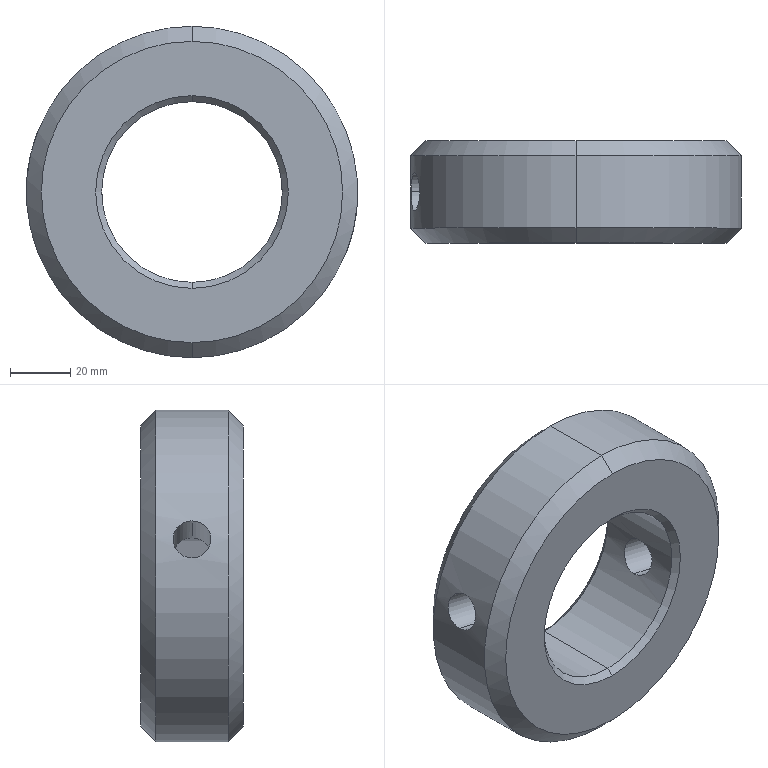Part | SolidWorks | features Chamfer 2, 3DProfileFeature 1, Extrusion 1, HoleWzd 1 | 1 solid | 18 faces | box 110 x 34 x 110 mm | volume 211578 mm3 | cone 8 | cylinder 8 | plane 2 | commonest cylinder face diameters 12.6 x4 60 x2 110 x2
STEP:
#1=CARTESIAN_POINT('',(0.,32.,-30.));
#2=VERTEX_POINT('',#1);
#3=CARTESIAN_POINT('',(0.,32.,30.));
#4=VERTEX_POINT('',#3);
#5=CARTESIAN_POINT('',(0.,32.,0.));
#6=DIRECTION('',(0.,1.,0.));
#7=DIRECTION('',(0.,0.,1.));
#8=AXIS2_PLACEMENT_3D('',#5,#6,#7);
#9=CIRCLE('',#8,30.);
#10=EDGE_CURVE('',#2,#4,#9,.T.);
#11=ORIENTED_EDGE('',*,*,#10,.F.);
#12=CARTESIAN_POINT('',(0.,34.,-32.));
#13=VERTEX_POINT('',#12);
#14=CARTESIAN_POINT('',(0.,32.,-30.));
#15=DIRECTION('',(0.,0.7071,-0.7071));
#16=VECTOR('',#15,1000.);
#17=LINE('',#14,#16);
#18=EDGE_CURVE('',#2,#13,#17,.T.);
#19=ORIENTED_EDGE('',*,*,#18,.T.);
#20=CARTESIAN_POINT('',(0.,34.,32.));
#21=VERTEX_POINT('',#20);
#22=CARTESIAN_POINT('',(0.,34.,0.));
#23=DIRECTION('',(0.,-1.,0.));
#24=DIRECTION('',(0.,0.,1.));
#25=AXIS2_PLACEMENT_3D('',#22,#23,#24);
#26=CIRCLE('',#25,32.);
#27=EDGE_CURVE('',#21,#13,#26,.T.);
#28=ORIENTED_EDGE('',*,*,#27,.F.);
#29=CARTESIAN_POINT('',(0.,32.,30.));
#30=DIRECTION('',(0.,0.7071,0.7071));
#31=VECTOR('',#30,1000.);
#32=LINE('',#29,#31);
#33=EDGE_CURVE('',#4,#21,#32,.T.);
#34=ORIENTED_EDGE('',*,*,#33,.F.);
#35=EDGE_LOOP('',(#11,#19,#28,#34));
#36=FACE_OUTER_BOUND('',#35,.T.);
#37=CARTESIAN_POINT('',(0.,32.,0.));
#38=DIRECTION('',(0.,1.,0.));
#39=DIRECTION('',(0.,0.,1.));
#40=AXIS2_PLACEMENT_3D('',#37,#38,#39);
#41=CONICAL_SURFACE('',#40,30.,0.7854);
#42=ADVANCED_FACE('',(#36),#41,.F.);
#43=CARTESIAN_POINT('',(0.,2.,30.));
#44=VERTEX_POINT('',#43);
#45=CARTESIAN_POINT('',(0.,2.,-30.));
#46=VERTEX_POINT('',#45);
#47=CARTESIAN_POINT('',(0.,2.,0.));
#48=DIRECTION('',(0.,-1.,0.));
#49=DIRECTION('',(0.,0.,1.));
#50=AXIS2_PLACEMENT_3D('',#47,#48,#49);
#51=CIRCLE('',#50,30.);
#52=EDGE_CURVE('',#44,#46,#51,.T.);
#53=ORIENTED_EDGE('',*,*,#52,.F.);
#54=CARTESIAN_POINT('',(0.,0.,32.));
#55=VERTEX_POINT('',#54);
#56=CARTESIAN_POINT('',(0.,0.,32.));
#57=DIRECTION('',(0.,-0.7071,0.7071));
#58=VECTOR('',#57,1000.);
#59=LINE('',#56,#58);
#60=EDGE_CURVE('',#44,#55,#59,.T.);
#61=ORIENTED_EDGE('',*,*,#60,.T.);
#62=CARTESIAN_POINT('',(0.,0.,-32.));
#63=VERTEX_POINT('',#62);
#64=CARTESIAN_POINT('',(0.,0.,0.));
#65=DIRECTION('',(0.,1.,0.));
#66=DIRECTION('',(0.,0.,1.));
#67=AXIS2_PLACEMENT_3D('',#64,#65,#66);
#68=CIRCLE('',#67,32.);
#69=EDGE_CURVE('',#63,#55,#68,.T.);
#70=ORIENTED_EDGE('',*,*,#69,.F.);
#71=CARTESIAN_POINT('',(0.,0.,-32.));
#72=DIRECTION('',(0.,-0.7071,-0.7071));
#73=VECTOR('',#72,1000.);
#74=LINE('',#71,#73);
#75=EDGE_CURVE('',#46,#63,#74,.T.);
#76=ORIENTED_EDGE('',*,*,#75,.F.);
#77=EDGE_LOOP('',(#53,#61,#70,#76));
#78=FACE_OUTER_BOUND('',#77,.T.);
#79=CARTESIAN_POINT('',(0.,0.,0.));
#80=DIRECTION('',(0.,-1.,0.));
#81=DIRECTION('',(0.,0.,-1.));
#82=AXIS2_PLACEMENT_3D('',#79,#80,#81);
#83=CONICAL_SURFACE('',#82,32.,0.7854);
#84=ADVANCED_FACE('',(#78),#83,.F.);
#85=CARTESIAN_POINT('',(0.,34.,50.));
#86=VERTEX_POINT('',#85);
#87=CARTESIAN_POINT('',(0.,34.,-50.));
#88=VERTEX_POINT('',#87);
#89=CARTESIAN_POINT('',(0.,34.,0.));
#90=DIRECTION('',(0.,1.,0.));
#91=DIRECTION('',(0.,0.,1.));
#92=AXIS2_PLACEMENT_3D('',#89,#90,#91);
#93=CIRCLE('',#92,50.);
#94=EDGE_CURVE('',#86,#88,#93,.T.);
#95=ORIENTED_EDGE('',*,*,#94,.F.);
#96=CARTESIAN_POINT('',(0.,29.,55.));
#97=VERTEX_POINT('',#96);
#98=CARTESIAN_POINT('',(0.,34.,50.));
#99=DIRECTION('',(0.,-0.7071,0.7071));
#100=VECTOR('',#99,1000.);
#101=LINE('',#98,#100);
#102=EDGE_CURVE('',#86,#97,#101,.T.);
#103=ORIENTED_EDGE('',*,*,#102,.T.);
#104=CARTESIAN_POINT('',(0.,29.,-55.));
#105=VERTEX_POINT('',#104);
#106=CARTESIAN_POINT('',(0.,29.,0.));
#107=DIRECTION('',(0.,-1.,0.));
#108=DIRECTION('',(0.,0.,1.));
#109=AXIS2_PLACEMENT_3D('',#106,#107,#108);
#110=CIRCLE('',#109,55.);
#111=EDGE_CURVE('',#105,#97,#110,.T.);
#112=ORIENTED_EDGE('',*,*,#111,.F.);
#113=CARTESIAN_POINT('',(0.,34.,-50.));
#114=DIRECTION('',(0.,-0.7071,-0.7071));
#115=VECTOR('',#114,1000.);
#116=LINE('',#113,#115);
#117=EDGE_CURVE('',#88,#105,#116,.T.);
#118=ORIENTED_EDGE('',*,*,#117,.F.);
#119=EDGE_LOOP('',(#95,#103,#112,#118));
#120=FACE_OUTER_BOUND('',#119,.T.);
#121=CARTESIAN_POINT('',(0.,34.,0.));
#122=DIRECTION('',(0.,-1.,0.));
#123=DIRECTION('',(0.,0.,-1.));
#124=AXIS2_PLACEMENT_3D('',#121,#122,#123);
#125=CONICAL_SURFACE('',#124,50.,0.7854);
#126=ADVANCED_FACE('',(#120),#125,.T.);
#127=CARTESIAN_POINT('',(0.,0.,-50.));
#128=VERTEX_POINT('',#127);
#129=CARTESIAN_POINT('',(0.,0.,50.));
#130=VERTEX_POINT('',#129);
#131=CARTESIAN_POINT('',(0.,0.,0.));
#132=DIRECTION('',(0.,-1.,0.));
#133=DIRECTION('',(0.,0.,1.));
#134=AXIS2_PLACEMENT_3D('',#131,#132,#133);
#135=CIRCLE('',#134,50.);
#136=EDGE_CURVE('',#128,#130,#135,.T.);
#137=ORIENTED_EDGE('',*,*,#136,.F.);
#138=CARTESIAN_POINT('',(0.,5.,-55.));
#139=VERTEX_POINT('',#138);
#140=CARTESIAN_POINT('',(0.,5.,-55.));
#141=DIRECTION('',(0.,0.7071,-0.7071));
#142=VECTOR('',#141,1000.);
#143=LINE('',#140,#142);
#144=EDGE_CURVE('',#128,#139,#143,.T.);
#145=ORIENTED_EDGE('',*,*,#144,.T.);
#146=CARTESIAN_POINT('',(0.,5.,55.));
#147=VERTEX_POINT('',#146);
#148=CARTESIAN_POINT('',(0.,5.,0.));
#149=DIRECTION('',(0.,1.,0.));
#150=DIRECTION('',(0.,0.,1.));
#151=AXIS2_PLACEMENT_3D('',#148,#149,#150);
#152=CIRCLE('',#151,55.);
#153=EDGE_CURVE('',#147,#139,#152,.T.);
#154=ORIENTED_EDGE('',*,*,#153,.F.);
#155=CARTESIAN_POINT('',(0.,5.,55.));
#156=DIRECTION('',(0.,0.7071,0.7071));
#157=VECTOR('',#156,1000.);
#158=LINE('',#155,#157);
#159=EDGE_CURVE('',#130,#147,#158,.T.);
#160=ORIENTED_EDGE('',*,*,#159,.F.);
#161=EDGE_LOOP('',(#137,#145,#154,#160));
#162=FACE_OUTER_BOUND('',#161,.T.);
#163=CARTESIAN_POINT('',(0.,5.,0.));
#164=DIRECTION('',(0.,1.,0.));
#165=DIRECTION('',(0.,0.,1.));
#166=AXIS2_PLACEMENT_3D('',#163,#164,#165);
#167=CONICAL_SURFACE('',#166,55.,0.7854);
#168=ADVANCED_FACE('',(#162),#167,.T.);
#169=CARTESIAN_POINT('',(-51.87,17.,18.289));
#170=VERTEX_POINT('',#169);
#171=CARTESIAN_POINT('',(-54.671,17.,6.005));
#172=VERTEX_POINT('',#171);
#173=CARTESIAN_POINT('',(-51.87,17.,18.289));
#174=CARTESIAN_POINT('',(-51.87,16.589,18.289));
#175=CARTESIAN_POINT('',(-51.883,16.18,18.252));
#176=CARTESIAN_POINT('',(-51.924,15.57,18.137));
#177=CARTESIAN_POINT('',(-51.94,15.368,18.088));
#178=CARTESIAN_POINT('',(-51.98,14.973,17.975));
#179=CARTESIAN_POINT('',(-52.025,14.586,17.843));
#180=CARTESIAN_POINT('',(-52.082,14.215,17.676));
#181=CARTESIAN_POINT('',(-52.145,13.851,17.491));
#182=CARTESIAN_POINT('',(-52.179,13.672,17.389));
#183=CARTESIAN_POINT('',(-52.288,13.156,17.06));
#184=CARTESIAN_POINT('',(-52.369,12.839,16.811));
#185=CARTESIAN_POINT('',(-52.544,12.258,16.256));
#186=CARTESIAN_POINT('',(-52.639,11.992,15.946));
#187=CARTESIAN_POINT('',(-52.834,11.534,15.288));
#188=CARTESIAN_POINT('',(-52.933,11.341,14.94));
#189=CARTESIAN_POINT('',(-53.085,11.103,14.388));
#190=CARTESIAN_POINT('',(-53.136,11.032,14.198));
#191=CARTESIAN_POINT('',(-53.237,10.912,13.815));
#192=CARTESIAN_POINT('',(-53.287,10.862,13.622));
#193=CARTESIAN_POINT('',(-53.434,10.741,13.036));
#194=CARTESIAN_POINT('',(-53.53,10.7,12.638));
#195=CARTESIAN_POINT('',(-53.715,10.7,11.826));
#196=CARTESIAN_POINT('',(-53.802,10.74,11.426));
#197=CARTESIAN_POINT('',(-53.923,10.86,10.833));
#198=CARTESIAN_POINT('',(-53.962,10.91,10.637));
#199=CARTESIAN_POINT('',(-54.037,11.03,10.249));
#200=CARTESIAN_POINT('',(-54.073,11.1,10.055));
#201=CARTESIAN_POINT('',(-54.176,11.337,9.491));
#202=CARTESIAN_POINT('',(-54.237,11.53,9.134));
#203=CARTESIAN_POINT('',(-54.347,11.986,8.457));
#204=CARTESIAN_POINT('',(-54.396,12.252,8.136));
#205=CARTESIAN_POINT('',(-54.479,12.832,7.559));
#206=CARTESIAN_POINT('',(-54.514,13.149,7.299));
#207=CARTESIAN_POINT('',(-54.559,13.665,6.955));
#208=CARTESIAN_POINT('',(-54.572,13.844,6.848));
#209=CARTESIAN_POINT('',(-54.596,14.207,6.654));
#210=CARTESIAN_POINT('',(-54.607,14.392,6.566));
#211=CARTESIAN_POINT('',(-54.635,14.961,6.33));
#212=CARTESIAN_POINT('',(-54.649,15.357,6.209));
#213=CARTESIAN_POINT('',(-54.667,16.172,6.046));
#214=CARTESIAN_POINT('',(-54.671,16.583,6.005));
#215=CARTESIAN_POINT('',(-54.671,17.,6.005));
#216=B_SPLINE_CURVE_WITH_KNOTS('',3,(#173,#174,#175,#176,#177,#178,#179,#180,#181,#182,#183,#184,#185,#186,#187,#188,#189,#190,#191,#192,#193,#194,#195,#196,#197,#198,#199,#200,#201,#202,#203,#204,#205,#206,#207,#208,#209,#210,#211,#212,#213,#214,#215),.UNSPECIFIED.,.F.,.F.,(4,2,2,1,2,2,2,2,2,2,2,2,2,2,2,2,2,2,2,2,2,4),(0.01971,0.02094,0.02156,0.02218,0.02279,0.02341,0.02464,0.02587,0.0271,0.02772,0.02834,0.02957,0.0308,0.03141,0.03203,0.03326,0.03449,0.03573,0.03634,0.03696,0.03819,0.03942),.UNSPECIFIED.);
#217=EDGE_CURVE('',#170,#172,#216,.T.);
#218=ORIENTED_EDGE('',*,*,#217,.F.);
#219=CARTESIAN_POINT('',(-27.196,17.,12.663));
#220=VERTEX_POINT('',#219);
#221=CARTESIAN_POINT('',(55.024,17.,-6.085));
#222=DIRECTION('',(0.975,0.,-0.2223));
#223=VECTOR('',#222,1000.);
#224=LINE('',#221,#223);
#225=EDGE_CURVE('',#170,#220,#224,.T.);
#226=ORIENTED_EDGE('',*,*,#225,.T.);
#227=CARTESIAN_POINT('',(-29.998,17.,0.3785));
#228=VERTEX_POINT('',#227);
#229=CARTESIAN_POINT('',(-27.196,17.,12.663));
#230=CARTESIAN_POINT('',(-27.196,16.588,12.663));
#231=CARTESIAN_POINT('',(-27.214,16.178,12.626));
#232=CARTESIAN_POINT('',(-27.283,15.362,12.475));
#233=CARTESIAN_POINT('',(-27.335,14.966,12.363));
#234=CARTESIAN_POINT('',(-27.432,14.397,12.144));
#235=CARTESIAN_POINT('',(-27.469,14.212,12.062));
#236=CARTESIAN_POINT('',(-27.548,13.847,11.88));
#237=CARTESIAN_POINT('',(-27.591,13.669,11.78));
#238=CARTESIAN_POINT('',(-27.727,13.155,11.458));
#239=CARTESIAN_POINT('',(-27.827,12.838,11.215));
#240=CARTESIAN_POINT('',(-28.041,12.257,10.668));
#241=CARTESIAN_POINT('',(-28.155,11.992,10.363));
#242=CARTESIAN_POINT('',(-28.385,11.536,9.716));
#243=CARTESIAN_POINT('',(-28.501,11.342,9.372));
#244=CARTESIAN_POINT('',(-28.674,11.103,8.823));
#245=CARTESIAN_POINT('',(-28.731,11.033,8.635));
#246=CARTESIAN_POINT('',(-28.843,10.913,8.255));
#247=CARTESIAN_POINT('',(-28.951,10.812,7.871));
#248=CARTESIAN_POINT('',(-29.054,10.752,7.477));
#249=CARTESIAN_POINT('',(-29.154,10.711,7.078));
#250=CARTESIAN_POINT('',(-29.202,10.7,6.875));
#251=CARTESIAN_POINT('',(-29.341,10.7,6.267));
#252=CARTESIAN_POINT('',(-29.424,10.74,5.866));
#253=CARTESIAN_POINT('',(-29.571,10.901,5.071));
#254=CARTESIAN_POINT('',(-29.636,11.023,4.673));
#255=CARTESIAN_POINT('',(-29.746,11.338,3.918));
#256=CARTESIAN_POINT('',(-29.79,11.531,3.557));
#257=CARTESIAN_POINT('',(-29.846,11.875,3.042));
#258=CARTESIAN_POINT('',(-29.862,11.999,2.874));
#259=CARTESIAN_POINT('',(-29.892,12.26,2.554));
#260=CARTESIAN_POINT('',(-29.904,12.398,2.401));
#261=CARTESIAN_POINT('',(-29.937,12.832,1.963));
#262=CARTESIAN_POINT('',(-29.953,13.149,1.698));
#263=CARTESIAN_POINT('',(-29.976,13.838,1.23));
#264=CARTESIAN_POINT('',(-29.983,14.2,1.033));
#265=CARTESIAN_POINT('',(-29.99,14.769,0.792));
#266=CARTESIAN_POINT('',(-29.991,14.962,0.7208));
#267=CARTESIAN_POINT('',(-29.994,15.358,0.5974));
#268=CARTESIAN_POINT('',(-29.995,15.561,0.5451));
#269=CARTESIAN_POINT('',(-29.997,16.171,0.4206));
#270=CARTESIAN_POINT('',(-29.998,16.583,0.3785));
#271=CARTESIAN_POINT('',(-29.998,17.,0.3785));
#272=B_SPLINE_CURVE_WITH_KNOTS('',3,(#229,#230,#231,#232,#233,#234,#235,#236,#237,#238,#239,#240,#241,#242,#243,#244,#245,#246,#247,#248,#249,#250,#251,#252,#253,#254,#255,#256,#257,#258,#259,#260,#261,#262,#263,#264,#265,#266,#267,#268,#269,#270,#271),.UNSPECIFIED.,.F.,.F.,(4,2,2,2,2,2,2,2,2,1,2,2,2,2,2,2,2,2,2,2,2,4),(0.01975,0.02099,0.02222,0.02284,0.02345,0.02469,0.02592,0.02716,0.02777,0.02839,0.02901,0.02962,0.03086,0.03209,0.03333,0.03394,0.03456,0.0358,0.03703,0.03765,0.03826,0.0395),.UNSPECIFIED.);
#273=EDGE_CURVE('',#220,#228,#272,.T.);
#274=ORIENTED_EDGE('',*,*,#273,.T.);
#275=CARTESIAN_POINT('',(52.223,17.,-18.37));
#276=DIRECTION('',(0.975,0.,-0.2223));
#277=VECTOR('',#276,1000.);
#278=LINE('',#275,#277);
#279=EDGE_CURVE('',#172,#228,#278,.T.);
#280=ORIENTED_EDGE('',*,*,#279,.F.);
#281=EDGE_LOOP('',(#218,#226,#274,#280));
#282=FACE_OUTER_BOUND('',#281,.T.);
#283=CARTESIAN_POINT('',(53.624,17.,-12.228));
#284=DIRECTION('',(0.975,0.,-0.2223));
#285=DIRECTION('',(-0.2223,0.,-0.975));
#286=AXIS2_PLACEMENT_3D('',#283,#284,#285);
#287=CYLINDRICAL_SURFACE('',#286,6.3);
#288=ADVANCED_FACE('',(#282),#287,.F.);
#289=CARTESIAN_POINT('',(27.196,17.,-12.663));
#290=VERTEX_POINT('',#289);
#291=CARTESIAN_POINT('',(29.998,17.,-0.3785));
#292=VERTEX_POINT('',#291);
#293=CARTESIAN_POINT('',(27.196,17.,-12.663));
#294=CARTESIAN_POINT('',(27.196,16.582,-12.663));
#295=CARTESIAN_POINT('',(27.214,16.172,-12.625));
#296=CARTESIAN_POINT('',(27.266,15.567,-12.513));
#297=CARTESIAN_POINT('',(27.287,15.367,-12.467));
#298=CARTESIAN_POINT('',(27.338,14.971,-12.355));
#299=CARTESIAN_POINT('',(27.368,14.774,-12.289));
#300=CARTESIAN_POINT('',(27.466,14.202,-12.068));
#301=CARTESIAN_POINT('',(27.545,13.841,-11.887));
#302=CARTESIAN_POINT('',(27.726,13.157,-11.46));
#303=CARTESIAN_POINT('',(27.828,12.834,-11.211));
#304=CARTESIAN_POINT('',(28.042,12.255,-10.665));
#305=CARTESIAN_POINT('',(28.154,11.994,-10.366));
#306=CARTESIAN_POINT('',(28.386,11.534,-9.713));
#307=CARTESIAN_POINT('',(28.503,11.339,-9.365));
#308=CARTESIAN_POINT('',(28.674,11.103,-8.822));
#309=CARTESIAN_POINT('',(28.731,11.033,-8.636));
#310=CARTESIAN_POINT('',(28.842,10.913,-8.256));
#311=CARTESIAN_POINT('',(28.897,10.862,-8.061));
#312=CARTESIAN_POINT('',(29.058,10.74,-7.471));
#313=CARTESIAN_POINT('',(29.157,10.7,-7.074));
#314=CARTESIAN_POINT('',(29.34,10.7,-6.27));
#315=CARTESIAN_POINT('',(29.425,10.741,-5.86));
#316=CARTESIAN_POINT('',(29.572,10.903,-5.064));
#317=CARTESIAN_POINT('',(29.636,11.022,-4.675));
#318=CARTESIAN_POINT('',(29.718,11.26,-4.106));
#319=CARTESIAN_POINT('',(29.744,11.349,-3.918));
#320=CARTESIAN_POINT('',(29.789,11.544,-3.555));
#321=CARTESIAN_POINT('',(29.81,11.65,-3.379));
#322=CARTESIAN_POINT('',(29.865,11.991,-2.868));
#323=CARTESIAN_POINT('',(29.893,12.253,-2.547));
#324=CARTESIAN_POINT('',(29.938,12.839,-1.957));
#325=CARTESIAN_POINT('',(29.953,13.155,-1.694));
#326=CARTESIAN_POINT('',(29.97,13.666,-1.347));
#327=CARTESIAN_POINT('',(29.975,13.843,-1.239));
#328=CARTESIAN_POINT('',(29.982,14.208,-1.04));
#329=CARTESIAN_POINT('',(29.985,14.396,-0.9496));
#330=CARTESIAN_POINT('',(29.992,14.967,-0.7083));
#331=CARTESIAN_POINT('',(29.994,15.36,-0.5862));
#332=CARTESIAN_POINT('',(29.996,15.967,-0.4621));
#333=CARTESIAN_POINT('',(29.997,16.174,-0.4306));
#334=CARTESIAN_POINT('',(29.997,16.588,-0.3888));
#335=CARTESIAN_POINT('',(29.998,16.794,-0.3785));
#336=CARTESIAN_POINT('',(29.998,17.,-0.3785));
#337=B_SPLINE_CURVE_WITH_KNOTS('',3,(#293,#294,#295,#296,#297,#298,#299,#300,#301,#302,#303,#304,#305,#306,#307,#308,#309,#310,#311,#312,#313,#314,#315,#316,#317,#318,#319,#320,#321,#322,#323,#324,#325,#326,#327,#328,#329,#330,#331,#332,#333,#334,#335,#336),.UNSPECIFIED.,.F.,.F.,(4,2,2,2,2,2,2,2,2,2,2,2,2,2,2,2,2,2,2,2,2,4),(0.,0.001234,0.001852,0.002469,0.003703,0.004938,0.006172,0.007407,0.008024,0.008641,0.009876,0.01111,0.01234,0.01296,0.01358,0.01481,0.01605,0.01667,0.01728,0.01852,0.01913,0.01975),.UNSPECIFIED.);
#338=EDGE_CURVE('',#290,#292,#337,.T.);
#339=ORIENTED_EDGE('',*,*,#338,.T.);
#340=CARTESIAN_POINT('',(54.671,17.,-6.005));
#341=VERTEX_POINT('',#340);
#342=CARTESIAN_POINT('',(55.024,17.,-6.085));
#343=DIRECTION('',(0.975,0.,-0.2223));
#344=VECTOR('',#343,1000.);
#345=LINE('',#342,#344);
#346=EDGE_CURVE('',#292,#341,#345,.T.);
#347=ORIENTED_EDGE('',*,*,#346,.T.);
#348=CARTESIAN_POINT('',(51.87,17.,-18.289));
#349=VERTEX_POINT('',#348);
#350=CARTESIAN_POINT('',(51.87,17.,-18.289));
#351=CARTESIAN_POINT('',(51.87,16.583,-18.289));
#352=CARTESIAN_POINT('',(51.884,16.174,-18.251));
#353=CARTESIAN_POINT('',(51.924,15.569,-18.136));
#354=CARTESIAN_POINT('',(51.94,15.37,-18.089));
#355=CARTESIAN_POINT('',(51.98,14.974,-17.975));
#356=CARTESIAN_POINT('',(52.003,14.777,-17.908));
#357=CARTESIAN_POINT('',(52.08,14.205,-17.682));
#358=CARTESIAN_POINT('',(52.143,13.843,-17.498));
#359=CARTESIAN_POINT('',(52.287,13.159,-17.062));
#360=CARTESIAN_POINT('',(52.37,12.835,-16.808));
#361=CARTESIAN_POINT('',(52.545,12.254,-16.252));
#362=CARTESIAN_POINT('',(52.638,11.993,-15.948));
#363=CARTESIAN_POINT('',(52.785,11.648,-15.452));
#364=CARTESIAN_POINT('',(52.835,11.541,-15.28));
#365=CARTESIAN_POINT('',(52.935,11.347,-14.93));
#366=CARTESIAN_POINT('',(53.036,11.171,-14.572));
#367=CARTESIAN_POINT('',(53.136,11.032,-14.198));
#368=CARTESIAN_POINT('',(53.237,10.912,-13.816));
#369=CARTESIAN_POINT('',(53.287,10.862,-13.62));
#370=CARTESIAN_POINT('',(53.436,10.74,-13.029));
#371=CARTESIAN_POINT('',(53.532,10.7,-12.631));
#372=CARTESIAN_POINT('',(53.715,10.7,-11.829));
#373=CARTESIAN_POINT('',(53.803,10.741,-11.42));
#374=CARTESIAN_POINT('',(53.965,10.902,-10.628));
#375=CARTESIAN_POINT('',(54.039,11.021,-10.242));
#376=CARTESIAN_POINT('',(54.142,11.258,-9.679));
#377=CARTESIAN_POINT('',(54.175,11.347,-9.492));
#378=CARTESIAN_POINT('',(54.237,11.542,-9.133));
#379=CARTESIAN_POINT('',(54.266,11.648,-8.958));
#380=CARTESIAN_POINT('',(54.348,11.99,-8.452));
#381=CARTESIAN_POINT('',(54.396,12.251,-8.137));
#382=CARTESIAN_POINT('',(54.48,12.839,-7.553));
#383=CARTESIAN_POINT('',(54.515,13.157,-7.294));
#384=CARTESIAN_POINT('',(54.559,13.668,-6.953));
#385=CARTESIAN_POINT('',(54.572,13.844,-6.847));
#386=CARTESIAN_POINT('',(54.596,14.209,-6.652));
#387=CARTESIAN_POINT('',(54.607,14.398,-6.563));
#388=CARTESIAN_POINT('',(54.635,14.97,-6.327));
#389=CARTESIAN_POINT('',(54.649,15.363,-6.207));
#390=CARTESIAN_POINT('',(54.667,16.171,-6.046));
#391=CARTESIAN_POINT('',(54.671,16.589,-6.005));
#392=CARTESIAN_POINT('',(54.671,17.,-6.005));
#393=B_SPLINE_CURVE_WITH_KNOTS('',3,(#350,#351,#352,#353,#354,#355,#356,#357,#358,#359,#360,#361,#362,#363,#364,#365,#366,#367,#368,#369,#370,#371,#372,#373,#374,#375,#376,#377,#378,#379,#380,#381,#382,#383,#384,#385,#386,#387,#388,#389,#390,#391,#392),.UNSPECIFIED.,.F.,.F.,(4,2,2,2,2,2,2,2,1,2,2,2,2,2,2,2,2,2,2,2,2,4),(0.,0.001232,0.001848,0.002464,0.003696,0.004928,0.00616,0.006776,0.007392,0.008008,0.008624,0.009856,0.01109,0.01232,0.01294,0.01355,0.01478,0.01602,0.01663,0.01725,0.01848,0.01971),.UNSPECIFIED.);
#394=EDGE_CURVE('',#349,#341,#393,.T.);
#395=ORIENTED_EDGE('',*,*,#394,.F.);
#396=CARTESIAN_POINT('',(52.223,17.,-18.37));
#397=DIRECTION('',(0.975,0.,-0.2223));
#398=VECTOR('',#397,1000.);
#399=LINE('',#396,#398);
#400=EDGE_CURVE('',#290,#349,#399,.T.);
#401=ORIENTED_EDGE('',*,*,#400,.F.);
#402=EDGE_LOOP('',(#339,#347,#395,#401));
#403=FACE_OUTER_BOUND('',#402,.T.);
#404=CARTESIAN_POINT('',(53.624,17.,-12.228));
#405=DIRECTION('',(0.975,0.,-0.2223));
#406=DIRECTION('',(-0.2223,0.,-0.975));
#407=AXIS2_PLACEMENT_3D('',#404,#405,#406);
#408=CYLINDRICAL_SURFACE('',#407,6.3);
#409=ADVANCED_FACE('',(#403),#408,.F.);
#410=CARTESIAN_POINT('',(-29.998,17.,0.3785));
#411=CARTESIAN_POINT('',(-29.998,17.418,0.3785));
#412=CARTESIAN_POINT('',(-29.997,17.828,0.4206));
#413=CARTESIAN_POINT('',(-29.995,18.433,0.5438));
#414=CARTESIAN_POINT('',(-29.994,18.633,0.5949));
#415=CARTESIAN_POINT('',(-29.991,19.029,0.7178));
#416=CARTESIAN_POINT('',(-29.99,19.226,0.7898));
#417=CARTESIAN_POINT('',(-29.983,19.798,1.032));
#418=CARTESIAN_POINT('',(-29.976,20.159,1.229));
#419=CARTESIAN_POINT('',(-29.953,20.843,1.693));
#420=CARTESIAN_POINT('',(-29.937,21.166,1.961));
#421=CARTESIAN_POINT('',(-29.893,21.745,2.546));
#422=CARTESIAN_POINT('',(-29.865,22.006,2.864));
#423=CARTESIAN_POINT('',(-29.791,22.466,3.553));
#424=CARTESIAN_POINT('',(-29.746,22.661,3.917));
#425=CARTESIAN_POINT('',(-29.664,22.897,4.481));
#426=CARTESIAN_POINT('',(-29.635,22.967,4.673));
#427=CARTESIAN_POINT('',(-29.57,23.087,5.063));
#428=CARTESIAN_POINT('',(-29.535,23.138,5.263));
#429=CARTESIAN_POINT('',(-29.424,23.26,5.864));
#430=CARTESIAN_POINT('',(-29.341,23.3,6.265));
#431=CARTESIAN_POINT('',(-29.158,23.3,7.069));
#432=CARTESIAN_POINT('',(-29.057,23.259,7.475));
#433=CARTESIAN_POINT('',(-28.844,23.097,8.257));
#434=CARTESIAN_POINT('',(-28.733,22.978,8.635));
#435=CARTESIAN_POINT('',(-28.56,22.74,9.183));
#436=CARTESIAN_POINT('',(-28.502,22.651,9.364));
#437=CARTESIAN_POINT('',(-28.386,22.456,9.71));
#438=CARTESIAN_POINT('',(-28.328,22.35,9.877));
#439=CARTESIAN_POINT('',(-28.156,22.009,10.362));
#440=CARTESIAN_POINT('',(-28.042,21.747,10.664));
#441=CARTESIAN_POINT('',(-27.826,21.161,11.215));
#442=CARTESIAN_POINT('',(-27.726,20.845,11.459));
#443=CARTESIAN_POINT('',(-27.591,20.334,11.779));
#444=CARTESIAN_POINT('',(-27.549,20.157,11.878));
#445=CARTESIAN_POINT('',(-27.469,19.792,12.06));
#446=CARTESIAN_POINT('',(-27.433,19.604,12.143));
#447=CARTESIAN_POINT('',(-27.334,19.033,12.364));
#448=CARTESIAN_POINT('',(-27.284,18.64,12.475));
#449=CARTESIAN_POINT('',(-27.232,18.033,12.587));
#450=CARTESIAN_POINT('',(-27.218,17.826,12.616));
#451=CARTESIAN_POINT('',(-27.201,17.412,12.654));
#452=CARTESIAN_POINT('',(-27.196,17.206,12.663));
#453=CARTESIAN_POINT('',(-27.196,17.,12.663));
#454=B_SPLINE_CURVE_WITH_KNOTS('',3,(#410,#411,#412,#413,#414,#415,#416,#417,#418,#419,#420,#421,#422,#423,#424,#425,#426,#427,#428,#429,#430,#431,#432,#433,#434,#435,#436,#437,#438,#439,#440,#441,#442,#443,#444,#445,#446,#447,#448,#449,#450,#451,#452,#453),.UNSPECIFIED.,.F.,.F.,(4,2,2,2,2,2,2,2,2,2,2,2,2,2,2,2,2,2,2,2,2,4),(0.,0.001234,0.001852,0.002469,0.003703,0.004938,0.006172,0.007407,0.008024,0.008641,0.009876,0.01111,0.01234,0.01296,0.01358,0.01481,0.01605,0.01667,0.01728,0.01852,0.01913,0.01975),.UNSPECIFIED.);
#455=EDGE_CURVE('',#228,#220,#454,.T.);
#456=ORIENTED_EDGE('',*,*,#455,.F.);
#457=ORIENTED_EDGE('',*,*,#273,.F.);
#458=EDGE_LOOP('',(#456,#457));
#459=FACE_BOUND('',#458,.T.);
#460=ORIENTED_EDGE('',*,*,#10,.T.);
#461=CARTESIAN_POINT('',(0.,34.,30.));
#462=DIRECTION('',(0.,-1.,0.));
#463=VECTOR('',#462,1000.);
#464=LINE('',#461,#463);
#465=EDGE_CURVE('',#4,#44,#464,.T.);
#466=ORIENTED_EDGE('',*,*,#465,.T.);
#467=ORIENTED_EDGE('',*,*,#52,.T.);
#468=CARTESIAN_POINT('',(0.,34.,-30.));
#469=DIRECTION('',(0.,-1.,0.));
#470=VECTOR('',#469,1000.);
#471=LINE('',#468,#470);
#472=EDGE_CURVE('',#2,#46,#471,.T.);
#473=ORIENTED_EDGE('',*,*,#472,.F.);
#474=EDGE_LOOP('',(#460,#466,#467,#473));
#475=FACE_OUTER_BOUND('',#474,.T.);
#476=CARTESIAN_POINT('',(0.,34.,0.));
#477=DIRECTION('',(0.,-1.,0.));
#478=DIRECTION('',(0.,0.,-1.));
#479=AXIS2_PLACEMENT_3D('',#476,#477,#478);
#480=CYLINDRICAL_SURFACE('',#479,30.);
#481=ADVANCED_FACE('',(#459,#475),#480,.F.);
#482=ORIENTED_EDGE('',*,*,#394,.T.);
#483=CARTESIAN_POINT('',(54.671,17.,-6.005));
#484=CARTESIAN_POINT('',(54.671,17.411,-6.005));
#485=CARTESIAN_POINT('',(54.667,17.82,-6.045));
#486=CARTESIAN_POINT('',(54.653,18.43,-6.166));
#487=CARTESIAN_POINT('',(54.648,18.632,-6.216));
#488=CARTESIAN_POINT('',(54.634,19.027,-6.336));
#489=CARTESIAN_POINT('',(54.618,19.414,-6.475));
#490=CARTESIAN_POINT('',(54.597,19.785,-6.65));
#491=CARTESIAN_POINT('',(54.573,20.149,-6.843));
#492=CARTESIAN_POINT('',(54.559,20.328,-6.95));
#493=CARTESIAN_POINT('',(54.515,20.844,-7.294));
#494=CARTESIAN_POINT('',(54.48,21.161,-7.553));
#495=CARTESIAN_POINT('',(54.397,21.742,-8.129));
#496=CARTESIAN_POINT('',(54.348,22.008,-8.45));
#497=CARTESIAN_POINT('',(54.239,22.466,-9.127));
#498=CARTESIAN_POINT('',(54.178,22.659,-9.484));
#499=CARTESIAN_POINT('',(54.075,22.897,-10.047));
#500=CARTESIAN_POINT('',(54.039,22.968,-10.24));
#501=CARTESIAN_POINT('',(53.964,23.088,-10.629));
#502=CARTESIAN_POINT('',(53.925,23.138,-10.825));
#503=CARTESIAN_POINT('',(53.804,23.259,-11.417));
#504=CARTESIAN_POINT('',(53.717,23.3,-11.817));
#505=CARTESIAN_POINT('',(53.532,23.3,-12.629));
#506=CARTESIAN_POINT('',(53.436,23.26,-13.028));
#507=CARTESIAN_POINT('',(53.289,23.14,-13.614));
#508=CARTESIAN_POINT('',(53.239,23.09,-13.807));
#509=CARTESIAN_POINT('',(53.138,22.97,-14.19));
#510=CARTESIAN_POINT('',(53.087,22.9,-14.38));
#511=CARTESIAN_POINT('',(52.935,22.663,-14.933));
#512=CARTESIAN_POINT('',(52.836,22.47,-15.281));
#513=CARTESIAN_POINT('',(52.641,22.014,-15.939));
#514=CARTESIAN_POINT('',(52.546,21.748,-16.25));
#515=CARTESIAN_POINT('',(52.37,21.168,-16.806));
#516=CARTESIAN_POINT('',(52.289,20.851,-17.055));
#517=CARTESIAN_POINT('',(52.18,20.335,-17.385));
#518=CARTESIAN_POINT('',(52.146,20.156,-17.487));
#519=CARTESIAN_POINT('',(52.084,19.793,-17.672));
#520=CARTESIAN_POINT('',(52.055,19.608,-17.756));
#521=CARTESIAN_POINT('',(51.978,19.039,-17.981));
#522=CARTESIAN_POINT('',(51.938,18.643,-18.096));
#523=CARTESIAN_POINT('',(51.884,17.828,-18.251));
#524=CARTESIAN_POINT('',(51.87,17.417,-18.289));
#525=CARTESIAN_POINT('',(51.87,17.,-18.289));
#526=B_SPLINE_CURVE_WITH_KNOTS('',3,(#483,#484,#485,#486,#487,#488,#489,#490,#491,#492,#493,#494,#495,#496,#497,#498,#499,#500,#501,#502,#503,#504,#505,#506,#507,#508,#509,#510,#511,#512,#513,#514,#515,#516,#517,#518,#519,#520,#521,#522,#523,#524,#525),.UNSPECIFIED.,.F.,.F.,(4,2,2,1,2,2,2,2,2,2,2,2,2,2,2,2,2,2,2,2,2,4),(0.01971,0.02094,0.02156,0.02218,0.02279,0.02341,0.02464,0.02587,0.0271,0.02772,0.02834,0.02957,0.0308,0.03141,0.03203,0.03326,0.03449,0.03573,0.03634,0.03696,0.03819,0.03942),.UNSPECIFIED.);
#527=EDGE_CURVE('',#341,#349,#526,.T.);
#528=ORIENTED_EDGE('',*,*,#527,.T.);
#529=EDGE_LOOP('',(#482,#528));
#530=FACE_BOUND('',#529,.T.);
#531=ORIENTED_EDGE('',*,*,#111,.T.);
#532=CARTESIAN_POINT('',(0.,34.,55.));
#533=DIRECTION('',(0.,-1.,0.));
#534=VECTOR('',#533,1000.);
#535=LINE('',#532,#534);
#536=EDGE_CURVE('',#97,#147,#535,.T.);
#537=ORIENTED_EDGE('',*,*,#536,.T.);
#538=ORIENTED_EDGE('',*,*,#153,.T.);
#539=CARTESIAN_POINT('',(0.,34.,-55.));
#540=DIRECTION('',(0.,-1.,0.));
#541=VECTOR('',#540,1000.);
#542=LINE('',#539,#541);
#543=EDGE_CURVE('',#105,#139,#542,.T.);
#544=ORIENTED_EDGE('',*,*,#543,.F.);
#545=EDGE_LOOP('',(#531,#537,#538,#544));
#546=FACE_OUTER_BOUND('',#545,.T.);
#547=CARTESIAN_POINT('',(0.,34.,0.));
#548=DIRECTION('',(0.,-1.,0.));
#549=DIRECTION('',(0.,0.,-1.));
#550=AXIS2_PLACEMENT_3D('',#547,#548,#549);
#551=CYLINDRICAL_SURFACE('',#550,55.);
#552=ADVANCED_FACE('',(#530,#546),#551,.T.);
#553=ORIENTED_EDGE('',*,*,#27,.T.);
#554=CARTESIAN_POINT('',(0.,34.,0.));
#555=DIRECTION('',(0.,-1.,0.));
#556=DIRECTION('',(0.,0.,1.));
#557=AXIS2_PLACEMENT_3D('',#554,#555,#556);
#558=CIRCLE('',#557,32.);
#559=EDGE_CURVE('',#13,#21,#558,.T.);
#560=ORIENTED_EDGE('',*,*,#559,.T.);
#561=EDGE_LOOP('',(#553,#560));
#562=FACE_BOUND('',#561,.T.);
#563=CARTESIAN_POINT('',(0.,34.,0.));
#564=DIRECTION('',(0.,1.,0.));
#565=DIRECTION('',(0.,0.,1.));
#566=AXIS2_PLACEMENT_3D('',#563,#564,#565);
#567=CIRCLE('',#566,50.);
#568=EDGE_CURVE('',#88,#86,#567,.T.);
#569=ORIENTED_EDGE('',*,*,#568,.T.);
#570=ORIENTED_EDGE('',*,*,#94,.T.);
#571=EDGE_LOOP('',(#569,#570));
#572=FACE_OUTER_BOUND('',#571,.T.);
#573=CARTESIAN_POINT('',(0.,34.,0.));
#574=DIRECTION('',(0.,1.,0.));
#575=DIRECTION('',(0.,0.,1.));
#576=AXIS2_PLACEMENT_3D('',#573,#574,#575);
#577=PLANE('',#576);
#578=ADVANCED_FACE('',(#562,#572),#577,.T.);
#579=ORIENTED_EDGE('',*,*,#69,.T.);
#580=CARTESIAN_POINT('',(0.,0.,0.));
#581=DIRECTION('',(0.,1.,0.));
#582=DIRECTION('',(0.,0.,1.));
#583=AXIS2_PLACEMENT_3D('',#580,#581,#582);
#584=CIRCLE('',#583,32.);
#585=EDGE_CURVE('',#55,#63,#584,.T.);
#586=ORIENTED_EDGE('',*,*,#585,.T.);
#587=EDGE_LOOP('',(#579,#586));
#588=FACE_BOUND('',#587,.T.);
#589=CARTESIAN_POINT('',(0.,0.,0.));
#590=DIRECTION('',(0.,-1.,0.));
#591=DIRECTION('',(0.,0.,1.));
#592=AXIS2_PLACEMENT_3D('',#589,#590,#591);
#593=CIRCLE('',#592,50.);
#594=EDGE_CURVE('',#130,#128,#593,.T.);
#595=ORIENTED_EDGE('',*,*,#594,.T.);
#596=ORIENTED_EDGE('',*,*,#136,.T.);
#597=EDGE_LOOP('',(#595,#596));
#598=FACE_OUTER_BOUND('',#597,.T.);
#599=CARTESIAN_POINT('',(0.,0.,0.));
#600=DIRECTION('',(0.,1.,0.));
#601=DIRECTION('',(0.,0.,1.));
#602=AXIS2_PLACEMENT_3D('',#599,#600,#601);
#603=PLANE('',#602);
#604=ADVANCED_FACE('',(#588,#598),#603,.F.);
#605=ORIENTED_EDGE('',*,*,#536,.F.);
#606=CARTESIAN_POINT('',(0.,29.,0.));
#607=DIRECTION('',(0.,-1.,0.));
#608=DIRECTION('',(0.,0.,1.));
#609=AXIS2_PLACEMENT_3D('',#606,#607,#608);
#610=CIRCLE('',#609,55.);
#611=EDGE_CURVE('',#97,#105,#610,.T.);
#612=ORIENTED_EDGE('',*,*,#611,.T.);
#613=ORIENTED_EDGE('',*,*,#543,.T.);
#614=CARTESIAN_POINT('',(0.,5.,0.));
#615=DIRECTION('',(0.,1.,0.));
#616=DIRECTION('',(0.,0.,1.));
#617=AXIS2_PLACEMENT_3D('',#614,#615,#616);
#618=CIRCLE('',#617,55.);
#619=EDGE_CURVE('',#139,#147,#618,.T.);
#620=ORIENTED_EDGE('',*,*,#619,.T.);
#621=EDGE_LOOP('',(#605,#612,#613,#620));
#622=FACE_OUTER_BOUND('',#621,.T.);
#623=CARTESIAN_POINT('',(-54.671,17.,6.005));
#624=CARTESIAN_POINT('',(-54.671,17.417,6.005));
#625=CARTESIAN_POINT('',(-54.667,17.826,6.046));
#626=CARTESIAN_POINT('',(-54.653,18.431,6.166));
#627=CARTESIAN_POINT('',(-54.648,18.63,6.216));
#628=CARTESIAN_POINT('',(-54.634,19.026,6.336));
#629=CARTESIAN_POINT('',(-54.626,19.223,6.406));
#630=CARTESIAN_POINT('',(-54.598,19.795,6.643));
#631=CARTESIAN_POINT('',(-54.574,20.157,6.836));
#632=CARTESIAN_POINT('',(-54.515,20.841,7.292));
#633=CARTESIAN_POINT('',(-54.479,21.165,7.557));
#634=CARTESIAN_POINT('',(-54.396,21.746,8.133));
#635=CARTESIAN_POINT('',(-54.348,22.007,8.448));
#636=CARTESIAN_POINT('',(-54.266,22.352,8.959));
#637=CARTESIAN_POINT('',(-54.236,22.459,9.135));
#638=CARTESIAN_POINT('',(-54.175,22.653,9.494));
#639=CARTESIAN_POINT('',(-54.11,22.829,9.86));
#640=CARTESIAN_POINT('',(-54.039,22.968,10.24));
#641=CARTESIAN_POINT('',(-53.964,23.088,10.628));
#642=CARTESIAN_POINT('',(-53.924,23.138,10.827));
#643=CARTESIAN_POINT('',(-53.802,23.26,11.425));
#644=CARTESIAN_POINT('',(-53.715,23.3,11.824));
#645=CARTESIAN_POINT('',(-53.533,23.3,12.626));
#646=CARTESIAN_POINT('',(-53.435,23.259,13.033));
#647=CARTESIAN_POINT('',(-53.238,23.098,13.817));
#648=CARTESIAN_POINT('',(-53.138,22.979,14.197));
#649=CARTESIAN_POINT('',(-52.986,22.742,14.749));
#650=CARTESIAN_POINT('',(-52.935,22.653,14.931));
#651=CARTESIAN_POINT('',(-52.834,22.458,15.282));
#652=CARTESIAN_POINT('',(-52.785,22.352,15.452));
#653=CARTESIAN_POINT('',(-52.639,22.01,15.944));
#654=CARTESIAN_POINT('',(-52.546,21.749,16.249));
#655=CARTESIAN_POINT('',(-52.368,21.161,16.812));
#656=CARTESIAN_POINT('',(-52.288,20.843,17.06));
#657=CARTESIAN_POINT('',(-52.18,20.332,17.386));
#658=CARTESIAN_POINT('',(-52.146,20.156,17.487));
#659=CARTESIAN_POINT('',(-52.083,19.791,17.673));
#660=CARTESIAN_POINT('',(-52.054,19.602,17.758));
#661=CARTESIAN_POINT('',(-51.977,19.03,17.984));
#662=CARTESIAN_POINT('',(-51.937,18.637,18.097));
#663=CARTESIAN_POINT('',(-51.884,17.829,18.25));
#664=CARTESIAN_POINT('',(-51.87,17.411,18.289));
#665=CARTESIAN_POINT('',(-51.87,17.,18.289));
#666=B_SPLINE_CURVE_WITH_KNOTS('',3,(#623,#624,#625,#626,#627,#628,#629,#630,#631,#632,#633,#634,#635,#636,#637,#638,#639,#640,#641,#642,#643,#644,#645,#646,#647,#648,#649,#650,#651,#652,#653,#654,#655,#656,#657,#658,#659,#660,#661,#662,#663,#664,#665),.UNSPECIFIED.,.F.,.F.,(4,2,2,2,2,2,2,2,1,2,2,2,2,2,2,2,2,2,2,2,2,4),(0.,0.001232,0.001848,0.002464,0.003696,0.004928,0.00616,0.006776,0.007392,0.008008,0.008624,0.009856,0.01109,0.01232,0.01294,0.01355,0.01478,0.01602,0.01663,0.01725,0.01848,0.01971),.UNSPECIFIED.);
#667=EDGE_CURVE('',#172,#170,#666,.T.);
#668=ORIENTED_EDGE('',*,*,#667,.T.);
#669=ORIENTED_EDGE('',*,*,#217,.T.);
#670=EDGE_LOOP('',(#668,#669));
#671=FACE_BOUND('',#670,.T.);
#672=CARTESIAN_POINT('',(0.,34.,0.));
#673=DIRECTION('',(0.,-1.,0.));
#674=DIRECTION('',(0.,0.,-1.));
#675=AXIS2_PLACEMENT_3D('',#672,#673,#674);
#676=CYLINDRICAL_SURFACE('',#675,55.);
#677=ADVANCED_FACE('',(#622,#671),#676,.T.);
#678=ORIENTED_EDGE('',*,*,#465,.F.);
#679=CARTESIAN_POINT('',(0.,32.,0.));
#680=DIRECTION('',(0.,1.,0.));
#681=DIRECTION('',(0.,0.,1.));
#682=AXIS2_PLACEMENT_3D('',#679,#680,#681);
#683=CIRCLE('',#682,30.);
#684=EDGE_CURVE('',#4,#2,#683,.T.);
#685=ORIENTED_EDGE('',*,*,#684,.T.);
#686=ORIENTED_EDGE('',*,*,#472,.T.);
#687=CARTESIAN_POINT('',(0.,2.,0.));
#688=DIRECTION('',(0.,-1.,0.));
#689=DIRECTION('',(0.,0.,1.));
#690=AXIS2_PLACEMENT_3D('',#687,#688,#689);
#691=CIRCLE('',#690,30.);
#692=EDGE_CURVE('',#46,#44,#691,.T.);
#693=ORIENTED_EDGE('',*,*,#692,.T.);
#694=EDGE_LOOP('',(#678,#685,#686,#693));
#695=FACE_OUTER_BOUND('',#694,.T.);
#696=ORIENTED_EDGE('',*,*,#338,.F.);
#697=CARTESIAN_POINT('',(29.998,17.,-0.3785));
#698=CARTESIAN_POINT('',(29.998,17.412,-0.3785));
#699=CARTESIAN_POINT('',(29.997,17.822,-0.4194));
#700=CARTESIAN_POINT('',(29.994,18.638,-0.5855));
#701=CARTESIAN_POINT('',(29.992,19.034,-0.7087));
#702=CARTESIAN_POINT('',(29.985,19.603,-0.949));
#703=CARTESIAN_POINT('',(29.982,19.788,-1.039));
#704=CARTESIAN_POINT('',(29.975,20.153,-1.237));
#705=CARTESIAN_POINT('',(29.97,20.331,-1.346));
#706=CARTESIAN_POINT('',(29.953,20.845,-1.694));
#707=CARTESIAN_POINT('',(29.938,21.162,-1.957));
#708=CARTESIAN_POINT('',(29.894,21.743,-2.542));
#709=CARTESIAN_POINT('',(29.865,22.008,-2.867));
#710=CARTESIAN_POINT('',(29.791,22.464,-3.55));
#711=CARTESIAN_POINT('',(29.747,22.658,-3.91));
#712=CARTESIAN_POINT('',(29.664,22.897,-4.479));
#713=CARTESIAN_POINT('',(29.634,22.967,-4.674));
#714=CARTESIAN_POINT('',(29.57,23.087,-5.064));
#715=CARTESIAN_POINT('',(29.501,23.188,-5.458));
#716=CARTESIAN_POINT('',(29.423,23.248,-5.858));
#717=CARTESIAN_POINT('',(29.34,23.289,-6.26));
#718=CARTESIAN_POINT('',(29.296,23.3,-6.464));
#719=CARTESIAN_POINT('',(29.157,23.3,-7.072));
#720=CARTESIAN_POINT('',(29.058,23.26,-7.47));
#721=CARTESIAN_POINT('',(28.846,23.099,-8.25));
#722=CARTESIAN_POINT('',(28.733,22.977,-8.636));
#723=CARTESIAN_POINT('',(28.504,22.662,-9.364));
#724=CARTESIAN_POINT('',(28.388,22.469,-9.709));
#725=CARTESIAN_POINT('',(28.214,22.125,-10.197));
#726=CARTESIAN_POINT('',(28.156,22.001,-10.356));
#727=CARTESIAN_POINT('',(28.044,21.74,-10.657));
#728=CARTESIAN_POINT('',(27.989,21.602,-10.8));
#729=CARTESIAN_POINT('',(27.829,21.168,-11.209));
#730=CARTESIAN_POINT('',(27.728,20.851,-11.455));
#731=CARTESIAN_POINT('',(27.546,20.162,-11.886));
#732=CARTESIAN_POINT('',(27.467,19.8,-12.067));
#733=CARTESIAN_POINT('',(27.368,19.231,-12.287));
#734=CARTESIAN_POINT('',(27.339,19.038,-12.352));
#735=CARTESIAN_POINT('',(27.288,18.642,-12.464));
#736=CARTESIAN_POINT('',(27.266,18.439,-12.512));
#737=CARTESIAN_POINT('',(27.214,17.829,-12.625));
#738=CARTESIAN_POINT('',(27.196,17.417,-12.663));
#739=CARTESIAN_POINT('',(27.196,17.,-12.663));
#740=B_SPLINE_CURVE_WITH_KNOTS('',3,(#697,#698,#699,#700,#701,#702,#703,#704,#705,#706,#707,#708,#709,#710,#711,#712,#713,#714,#715,#716,#717,#718,#719,#720,#721,#722,#723,#724,#725,#726,#727,#728,#729,#730,#731,#732,#733,#734,#735,#736,#737,#738,#739),.UNSPECIFIED.,.F.,.F.,(4,2,2,2,2,2,2,2,2,1,2,2,2,2,2,2,2,2,2,2,2,4),(0.01975,0.02099,0.02222,0.02284,0.02345,0.02469,0.02592,0.02716,0.02777,0.02839,0.02901,0.02962,0.03086,0.03209,0.03333,0.03394,0.03456,0.0358,0.03703,0.03765,0.03826,0.0395),.UNSPECIFIED.);
#741=EDGE_CURVE('',#292,#290,#740,.T.);
#742=ORIENTED_EDGE('',*,*,#741,.F.);
#743=EDGE_LOOP('',(#696,#742));
#744=FACE_BOUND('',#743,.T.);
#745=CARTESIAN_POINT('',(0.,34.,0.));
#746=DIRECTION('',(0.,-1.,0.));
#747=DIRECTION('',(0.,0.,-1.));
#748=AXIS2_PLACEMENT_3D('',#745,#746,#747);
#749=CYLINDRICAL_SURFACE('',#748,30.);
#750=ADVANCED_FACE('',(#695,#744),#749,.F.);
#751=ORIENTED_EDGE('',*,*,#346,.F.);
#752=ORIENTED_EDGE('',*,*,#741,.T.);
#753=ORIENTED_EDGE('',*,*,#400,.T.);
#754=ORIENTED_EDGE('',*,*,#527,.F.);
#755=EDGE_LOOP('',(#751,#752,#753,#754));
#756=FACE_OUTER_BOUND('',#755,.T.);
#757=CARTESIAN_POINT('',(53.624,17.,-12.228));
#758=DIRECTION('',(0.975,0.,-0.2223));
#759=DIRECTION('',(-0.2223,0.,-0.975));
#760=AXIS2_PLACEMENT_3D('',#757,#758,#759);
#761=CYLINDRICAL_SURFACE('',#760,6.3);
#762=ADVANCED_FACE('',(#756),#761,.F.);
#763=ORIENTED_EDGE('',*,*,#225,.F.);
#764=ORIENTED_EDGE('',*,*,#667,.F.);
#765=ORIENTED_EDGE('',*,*,#279,.T.);
#766=ORIENTED_EDGE('',*,*,#455,.T.);
#767=EDGE_LOOP('',(#763,#764,#765,#766));
#768=FACE_OUTER_BOUND('',#767,.T.);
#769=CARTESIAN_POINT('',(53.624,17.,-12.228));
#770=DIRECTION('',(0.975,0.,-0.2223));
#771=DIRECTION('',(-0.2223,0.,-0.975));
#772=AXIS2_PLACEMENT_3D('',#769,#770,#771);
#773=CYLINDRICAL_SURFACE('',#772,6.3);
#774=ADVANCED_FACE('',(#768),#773,.F.);
#775=ORIENTED_EDGE('',*,*,#144,.F.);
#776=ORIENTED_EDGE('',*,*,#594,.F.);
#777=ORIENTED_EDGE('',*,*,#159,.T.);
#778=ORIENTED_EDGE('',*,*,#619,.F.);
#779=EDGE_LOOP('',(#775,#776,#777,#778));
#780=FACE_OUTER_BOUND('',#779,.T.);
#781=CARTESIAN_POINT('',(0.,5.,0.));
#782=DIRECTION('',(0.,1.,0.));
#783=DIRECTION('',(0.,0.,1.));
#784=AXIS2_PLACEMENT_3D('',#781,#782,#783);
#785=CONICAL_SURFACE('',#784,55.,0.7854);
#786=ADVANCED_FACE('',(#780),#785,.T.);
#787=ORIENTED_EDGE('',*,*,#102,.F.);
#788=ORIENTED_EDGE('',*,*,#568,.F.);
#789=ORIENTED_EDGE('',*,*,#117,.T.);
#790=ORIENTED_EDGE('',*,*,#611,.F.);
#791=EDGE_LOOP('',(#787,#788,#789,#790));
#792=FACE_OUTER_BOUND('',#791,.T.);
#793=CARTESIAN_POINT('',(0.,34.,0.));
#794=DIRECTION('',(0.,-1.,0.));
#795=DIRECTION('',(0.,0.,-1.));
#796=AXIS2_PLACEMENT_3D('',#793,#794,#795);
#797=CONICAL_SURFACE('',#796,50.,0.7854);
#798=ADVANCED_FACE('',(#792),#797,.T.);
#799=ORIENTED_EDGE('',*,*,#60,.F.);
#800=ORIENTED_EDGE('',*,*,#692,.F.);
#801=ORIENTED_EDGE('',*,*,#75,.T.);
#802=ORIENTED_EDGE('',*,*,#585,.F.);
#803=EDGE_LOOP('',(#799,#800,#801,#802));
#804=FACE_OUTER_BOUND('',#803,.T.);
#805=CARTESIAN_POINT('',(0.,0.,0.));
#806=DIRECTION('',(0.,-1.,0.));
#807=DIRECTION('',(0.,0.,-1.));
#808=AXIS2_PLACEMENT_3D('',#805,#806,#807);
#809=CONICAL_SURFACE('',#808,32.,0.7854);
#810=ADVANCED_FACE('',(#804),#809,.F.);
#811=ORIENTED_EDGE('',*,*,#18,.F.);
#812=ORIENTED_EDGE('',*,*,#684,.F.);
#813=ORIENTED_EDGE('',*,*,#33,.T.);
#814=ORIENTED_EDGE('',*,*,#559,.F.);
#815=EDGE_LOOP('',(#811,#812,#813,#814));
#816=FACE_OUTER_BOUND('',#815,.T.);
#817=CARTESIAN_POINT('',(0.,32.,0.));
#818=DIRECTION('',(0.,1.,0.));
#819=DIRECTION('',(0.,0.,1.));
#820=AXIS2_PLACEMENT_3D('',#817,#818,#819);
#821=CONICAL_SURFACE('',#820,30.,0.7854);
#822=ADVANCED_FACE('',(#816),#821,.F.);
#823=CLOSED_SHELL('',(#42,#84,#126,#168,#288,#409,#481,#552,#578,#604,#677,#750,#762,#774,#786,#798,#810,#822));
#824=MANIFOLD_SOLID_BREP('',#823);
#825=CARTESIAN_POINT('',(0.,0.,0.));
#826=DIRECTION('',(0.,0.,1.));
#827=DIRECTION('',(1.,0.,0.));
#828=AXIS2_PLACEMENT_3D('',#825,#826,#827);
#829=(LENGTH_UNIT()NAMED_UNIT(*)SI_UNIT(.MILLI.,.METRE.));
#830=UNCERTAINTY_MEASURE_WITH_UNIT(LENGTH_MEASURE(0.00001),#829,'','');
#831=(NAMED_UNIT(*)PLANE_ANGLE_UNIT()SI_UNIT($,.RADIAN.));
#832=(NAMED_UNIT(*)SI_UNIT($,.STERADIAN.)SOLID_ANGLE_UNIT());
#833=(GEOMETRIC_REPRESENTATION_CONTEXT(3)GLOBAL_UNCERTAINTY_ASSIGNED_CONTEXT((#830))GLOBAL_UNIT_ASSIGNED_CONTEXT((#829,#831,#832))REPRESENTATION_CONTEXT('',''));
#834=ADVANCED_BREP_SHAPE_REPRESENTATION('',(#824,#828),#833);